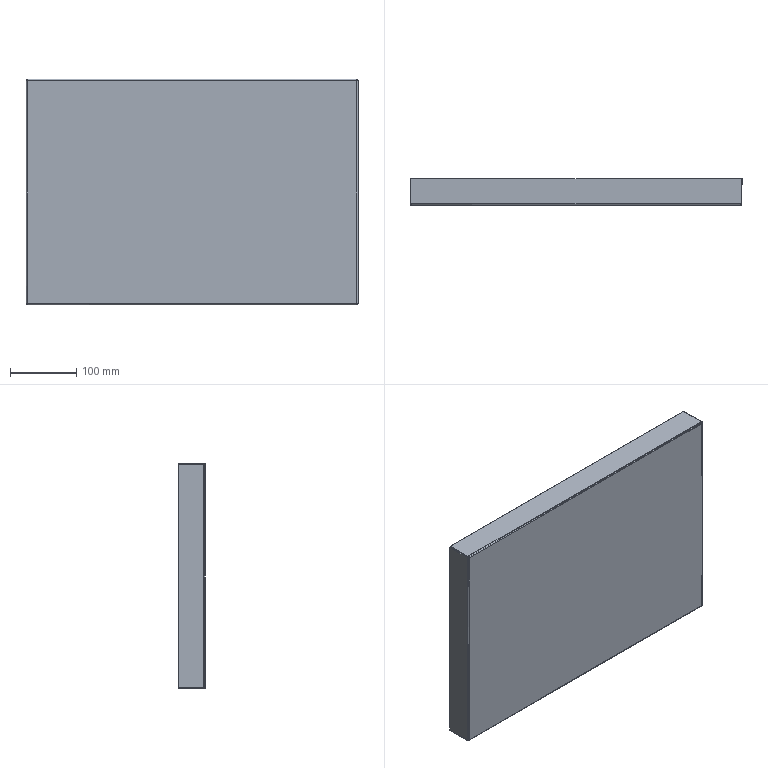Part | SolidWorks | features EdgeFlange 1, FlatPattern 1, SMBaseFlange 1, SheetMetal 1 | 1 solid | 38 faces | box 500 x 40 x 340 mm | volume 280304 mm3 | plane 22 | spline 8 | cylinder 8 | commonest cylinder face diameters 2 x4 4.4 x4